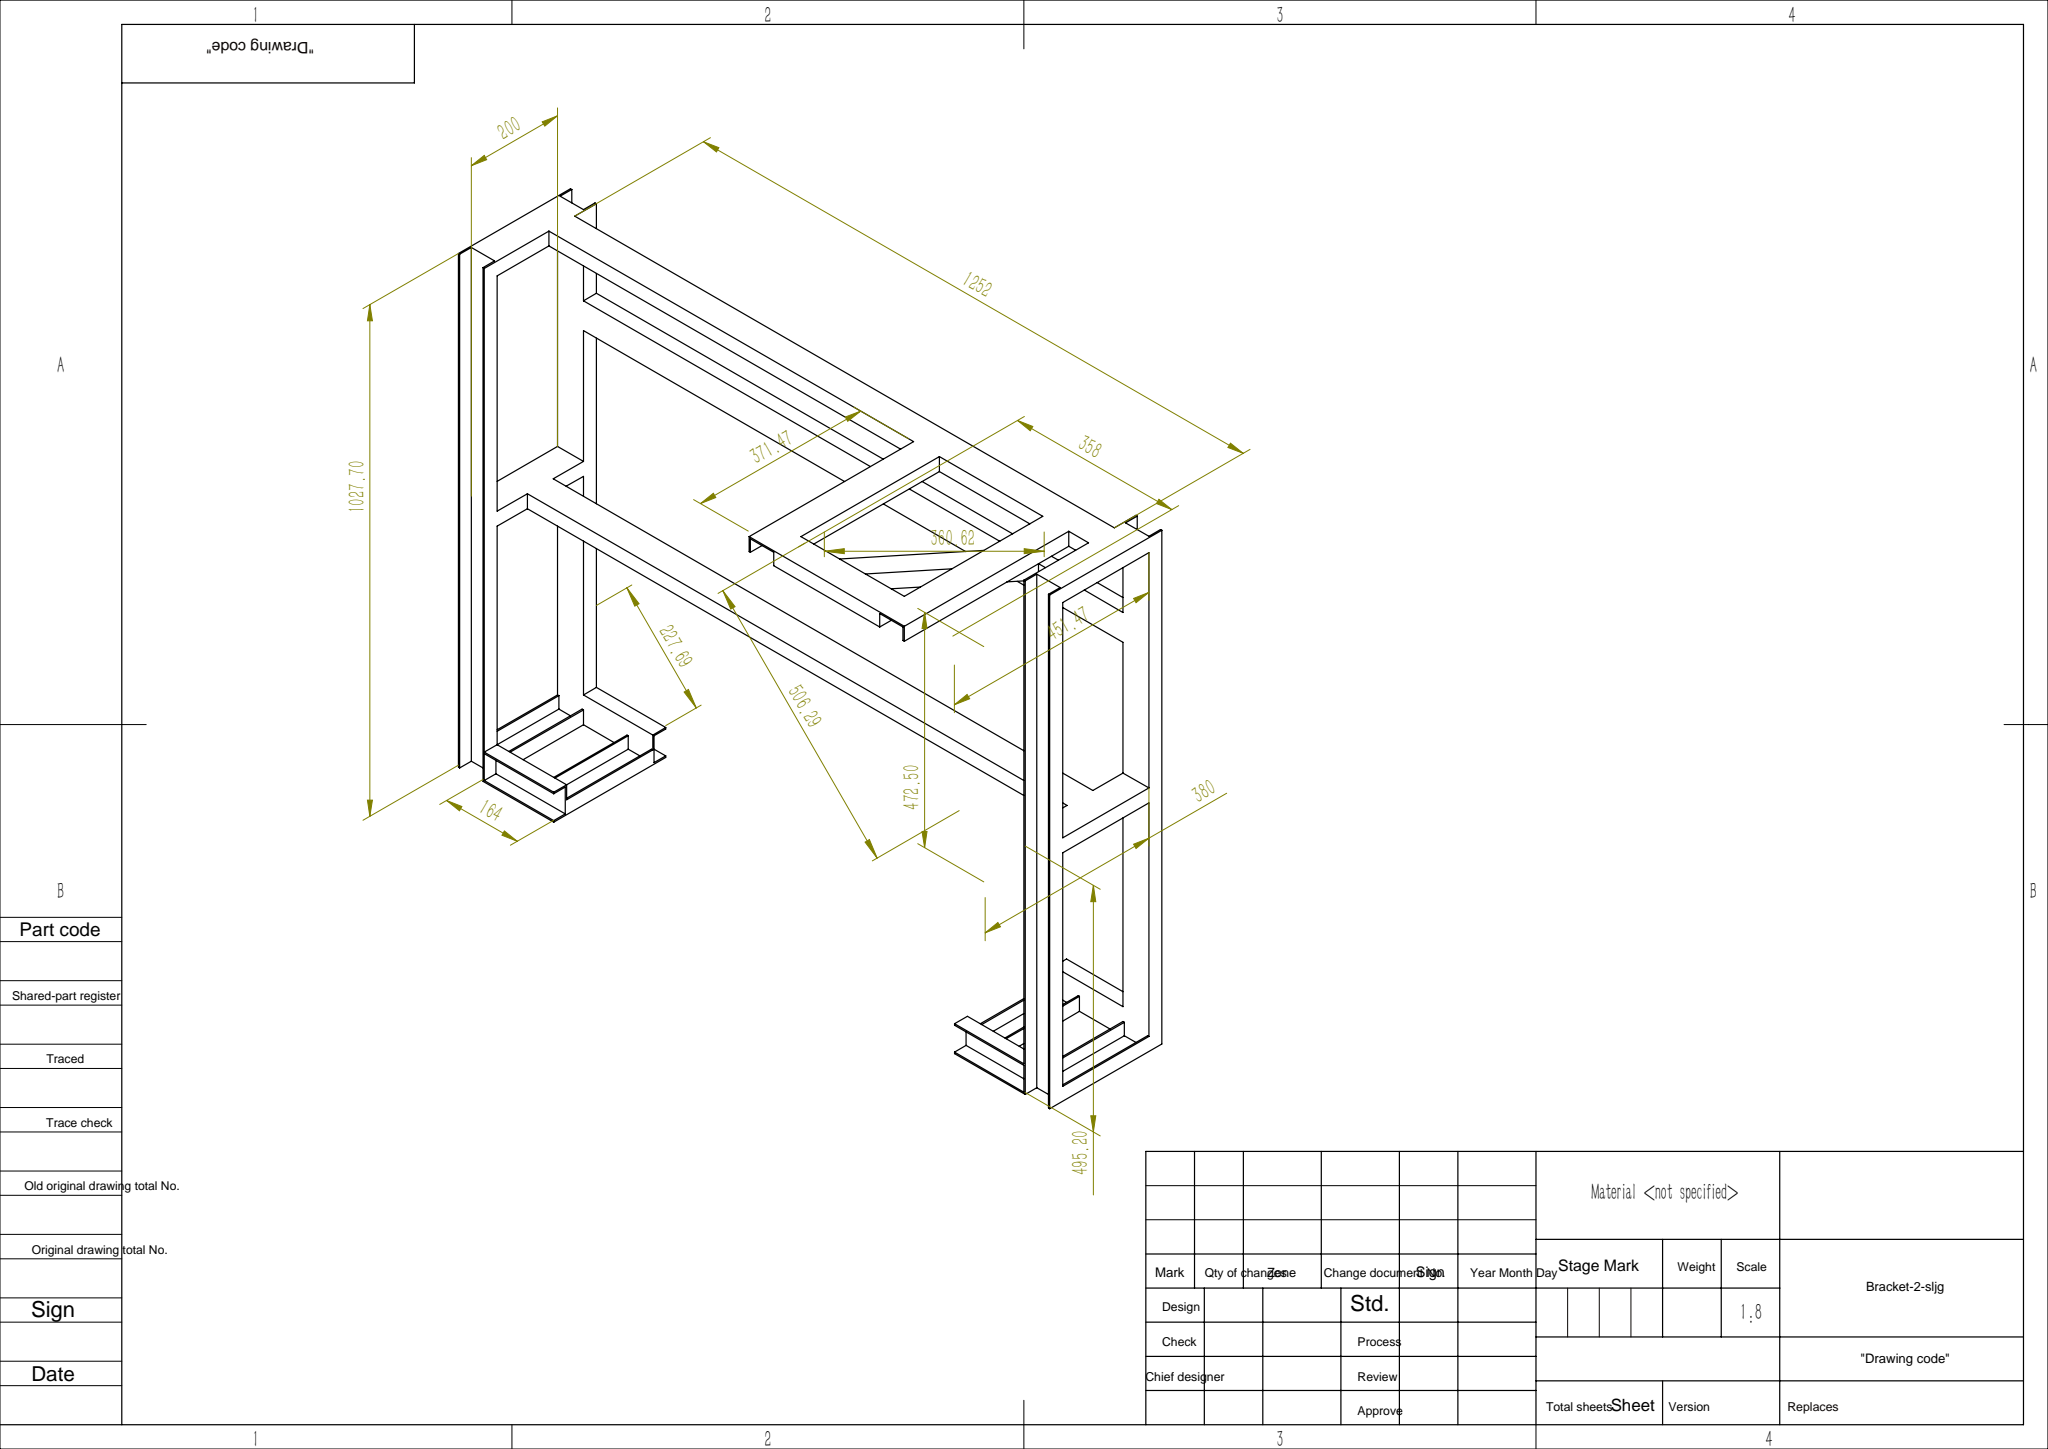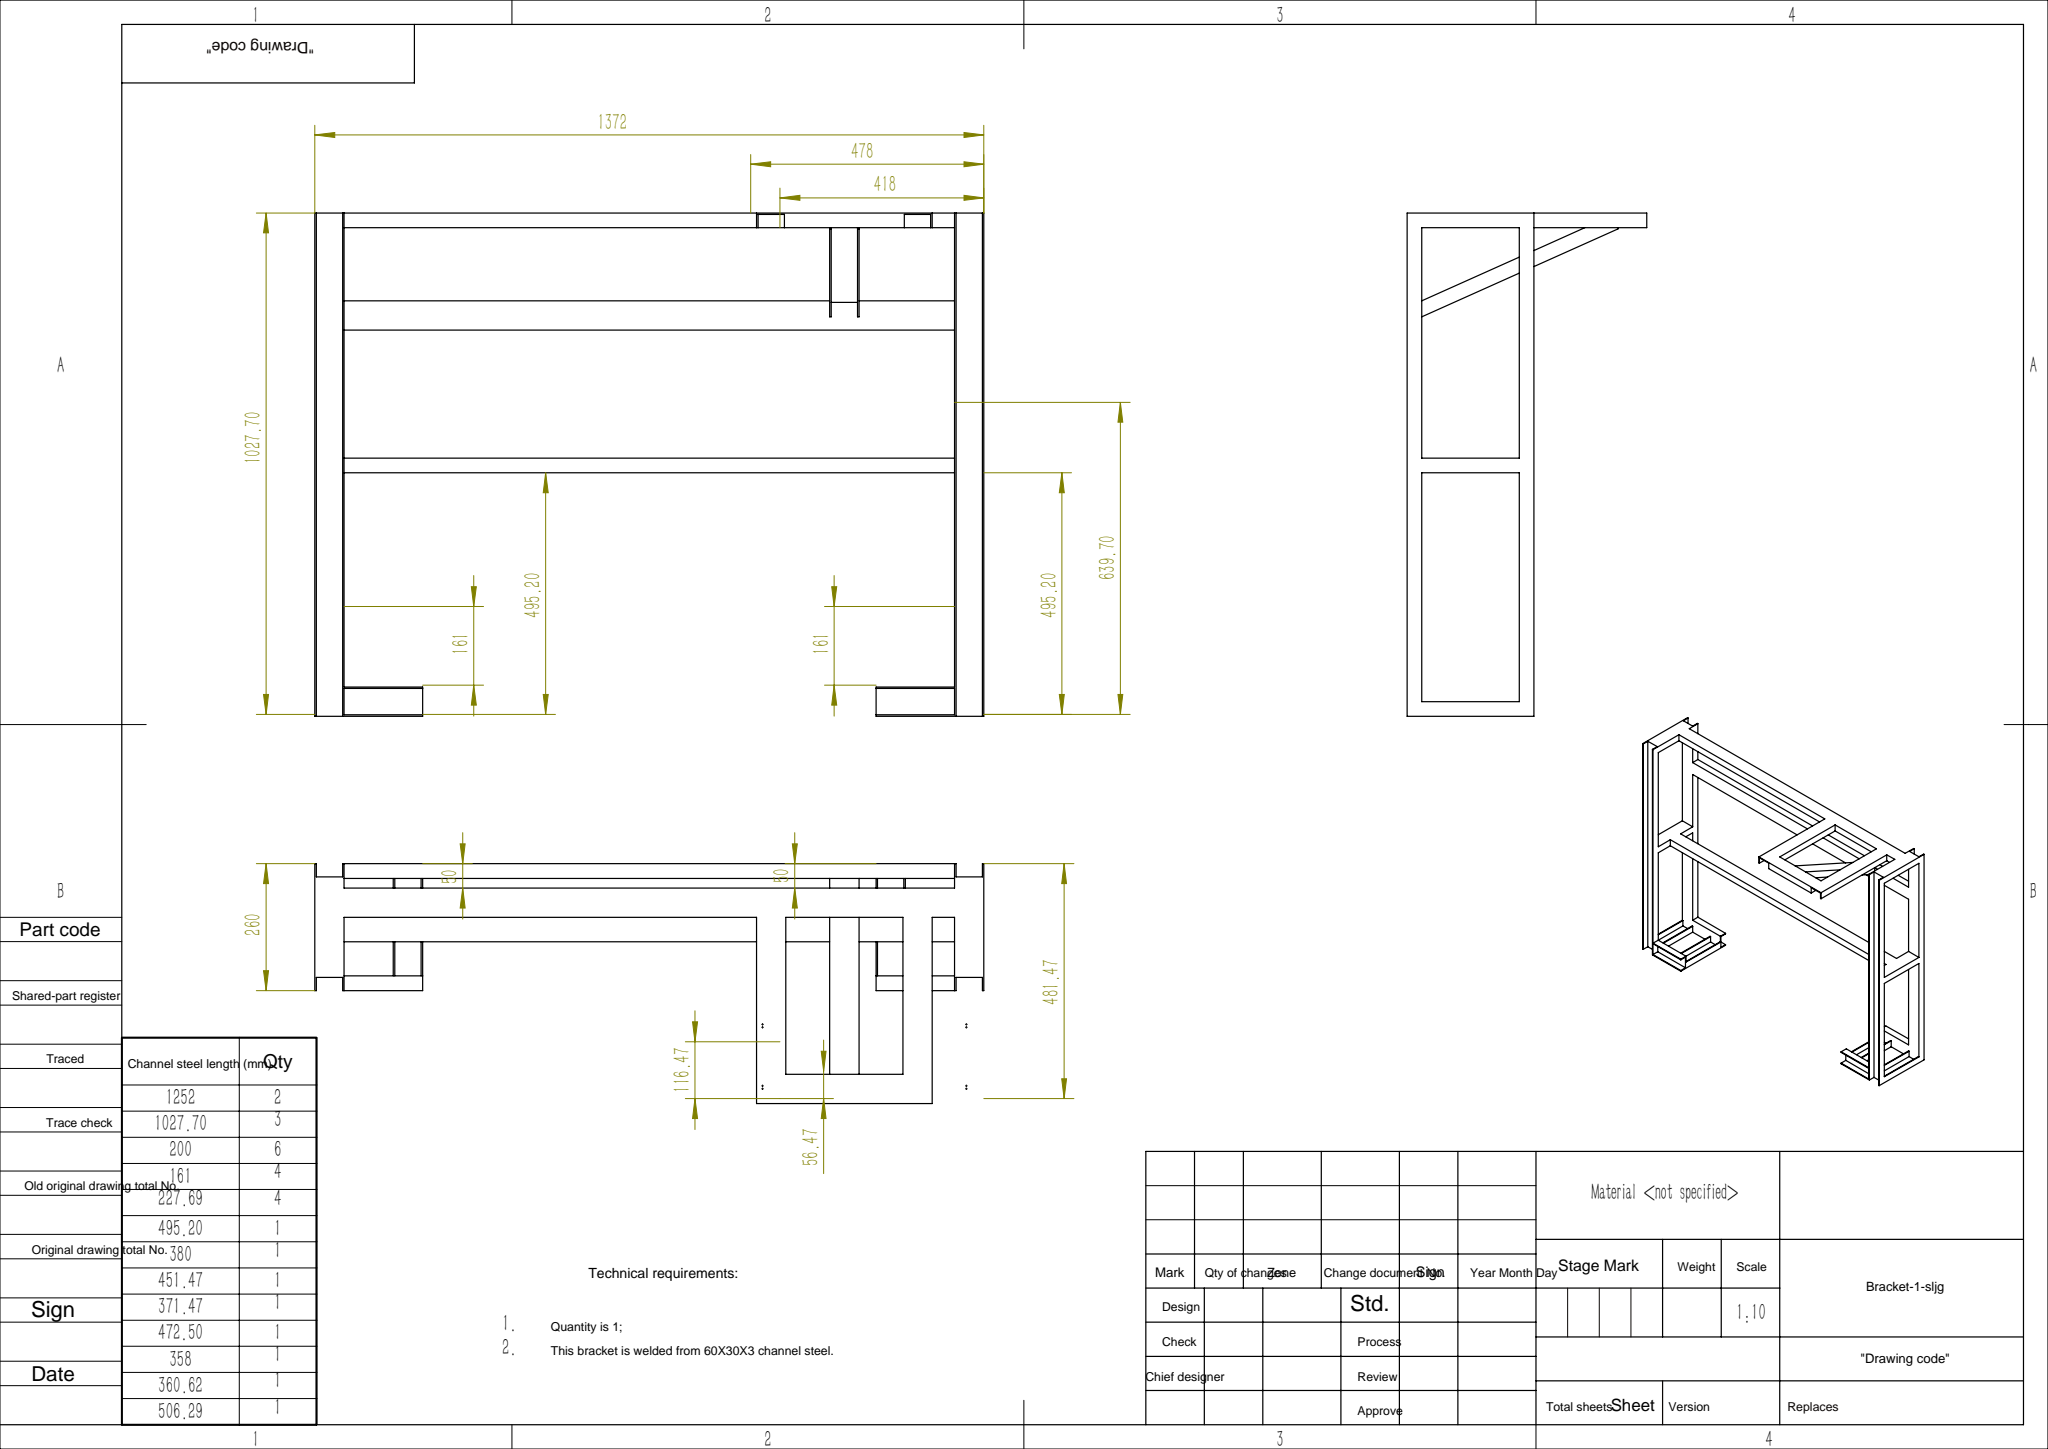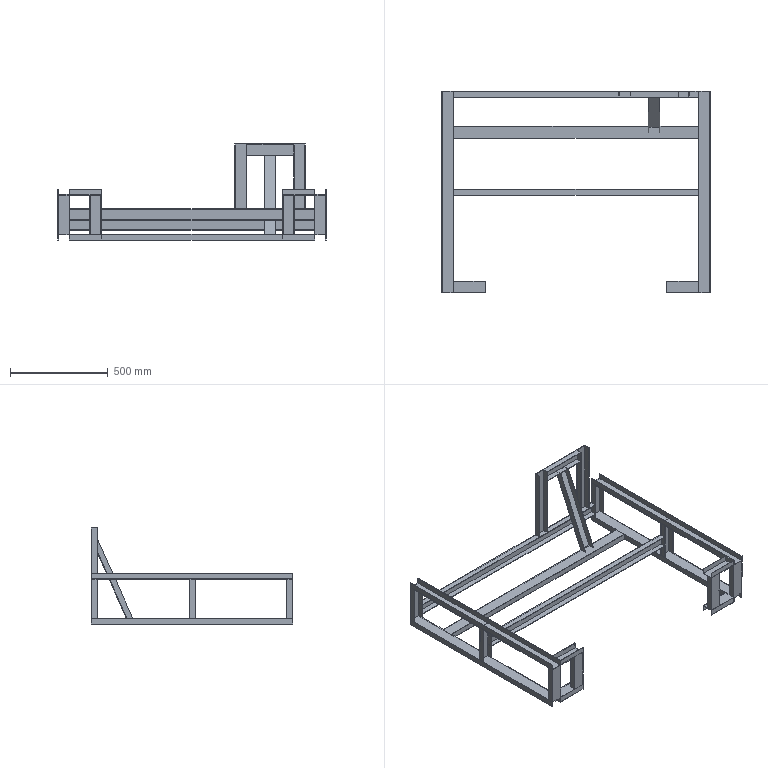Part | SolidWorks | features ICE 10, Extrusion 1, MirrorPattern 1, RefAxis 1, RefPoint 1 | 1 solid | 156 faces | box 1372 x 1032 x 491.47 mm | volume 3956578 mm3 | plane 156